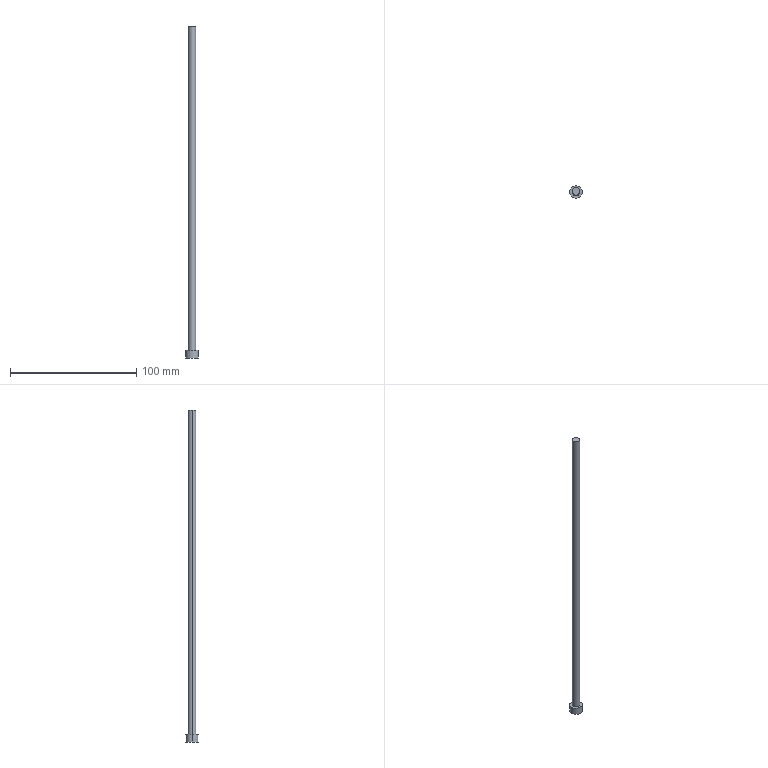Part | Creo | 1 solid | 7 faces | box 10 x 10 x 263.337 mm | volume 7747 mm3 | cylinder 4 | plane 3 | commonest cylinder face diameters 6 x2 10 x2
STEP:
#1=CARTESIAN_POINT('',(5.,161.,-32.663));
#2=VERTEX_POINT('',#1);
#3=CARTESIAN_POINT('',(11.,161.,-32.663));
#4=VERTEX_POINT('',#3);
#5=CARTESIAN_POINT('',(8.,161.,-32.663));
#6=DIRECTION('',(0.,0.,1.));
#7=DIRECTION('',(-1.,0.,0.));
#8=AXIS2_PLACEMENT_3D('',#5,#6,#7);
#9=CIRCLE('',#8,3.);
#10=EDGE_CURVE('',#2,#4,#9,.T.);
#11=ORIENTED_EDGE('',*,*,#10,.F.);
#12=CARTESIAN_POINT('',(8.,161.,-32.663));
#13=DIRECTION('',(0.,0.,1.));
#14=DIRECTION('',(1.,0.,0.));
#15=AXIS2_PLACEMENT_3D('',#12,#13,#14);
#16=CIRCLE('',#15,3.);
#17=EDGE_CURVE('',#4,#2,#16,.T.);
#18=ORIENTED_EDGE('',*,*,#17,.F.);
#19=EDGE_LOOP('',(#11,#18));
#20=FACE_OUTER_BOUND('',#19,.F.);
#21=CARTESIAN_POINT('',(-0.00000969,166.325,-32.663));
#22=DIRECTION('',(0.,0.,-1.));
#23=DIRECTION('',(0.,-1.,0.));
#24=AXIS2_PLACEMENT_3D('',#21,#22,#23);
#25=PLANE('',#24);
#26=ADVANCED_FACE('',(#20),#25,.F.);
#27=CARTESIAN_POINT('',(11.,161.,-290.));
#28=VERTEX_POINT('',#27);
#29=CARTESIAN_POINT('',(5.,161.,-290.));
#30=VERTEX_POINT('',#29);
#31=CARTESIAN_POINT('',(8.,161.,-290.));
#32=DIRECTION('',(0.,0.,-1.));
#33=DIRECTION('',(1.,0.,0.));
#34=AXIS2_PLACEMENT_3D('',#31,#32,#33);
#35=CIRCLE('',#34,3.);
#36=EDGE_CURVE('',#28,#30,#35,.T.);
#37=ORIENTED_EDGE('',*,*,#36,.T.);
#38=CARTESIAN_POINT('',(5.,161.,-290.));
#39=DIRECTION('',(0.,0.,1.));
#40=VECTOR('',#39,257.337);
#41=LINE('',#38,#40);
#42=EDGE_CURVE('',#30,#2,#41,.T.);
#43=ORIENTED_EDGE('',*,*,#42,.T.);
#44=ORIENTED_EDGE('',*,*,#10,.T.);
#45=CARTESIAN_POINT('',(11.,161.,-290.));
#46=DIRECTION('',(0.,0.,1.));
#47=VECTOR('',#46,257.337);
#48=LINE('',#45,#47);
#49=EDGE_CURVE('',#28,#4,#48,.T.);
#50=ORIENTED_EDGE('',*,*,#49,.F.);
#51=EDGE_LOOP('',(#37,#43,#44,#50));
#52=FACE_OUTER_BOUND('',#51,.F.);
#53=CARTESIAN_POINT('',(8.,161.,-351.071));
#54=DIRECTION('',(0.,0.,1.));
#55=DIRECTION('',(-1.,0.,0.));
#56=AXIS2_PLACEMENT_3D('',#53,#54,#55);
#57=CYLINDRICAL_SURFACE('',#56,3.);
#58=ADVANCED_FACE('',(#52),#57,.T.);
#59=CARTESIAN_POINT('',(13.,161.,-290.));
#60=VERTEX_POINT('',#59);
#61=CARTESIAN_POINT('',(3.,161.,-290.));
#62=VERTEX_POINT('',#61);
#63=CARTESIAN_POINT('',(8.,161.,-290.));
#64=DIRECTION('',(0.,0.,1.));
#65=DIRECTION('',(1.,0.,0.));
#66=AXIS2_PLACEMENT_3D('',#63,#64,#65);
#67=CIRCLE('',#66,5.);
#68=EDGE_CURVE('',#60,#62,#67,.T.);
#69=ORIENTED_EDGE('',*,*,#68,.F.);
#70=CARTESIAN_POINT('',(8.,161.,-290.));
#71=DIRECTION('',(0.,0.,1.));
#72=DIRECTION('',(-1.,0.,0.));
#73=AXIS2_PLACEMENT_3D('',#70,#71,#72);
#74=CIRCLE('',#73,5.);
#75=EDGE_CURVE('',#62,#60,#74,.T.);
#76=ORIENTED_EDGE('',*,*,#75,.F.);
#77=EDGE_LOOP('',(#69,#76));
#78=FACE_OUTER_BOUND('',#77,.F.);
#79=ORIENTED_EDGE('',*,*,#36,.F.);
#80=CARTESIAN_POINT('',(8.,161.,-290.));
#81=DIRECTION('',(0.,0.,-1.));
#82=DIRECTION('',(-1.,0.,0.));
#83=AXIS2_PLACEMENT_3D('',#80,#81,#82);
#84=CIRCLE('',#83,3.);
#85=EDGE_CURVE('',#30,#28,#84,.T.);
#86=ORIENTED_EDGE('',*,*,#85,.F.);
#87=EDGE_LOOP('',(#79,#86));
#88=FACE_BOUND('',#87,.F.);
#89=CARTESIAN_POINT('',(8.,161.,-290.));
#90=DIRECTION('',(0.,0.,1.));
#91=DIRECTION('',(-1.,0.,0.));
#92=AXIS2_PLACEMENT_3D('',#89,#90,#91);
#93=PLANE('',#92);
#94=ADVANCED_FACE('',(#78,#88),#93,.T.);
#95=ORIENTED_EDGE('',*,*,#85,.T.);
#96=ORIENTED_EDGE('',*,*,#49,.T.);
#97=ORIENTED_EDGE('',*,*,#17,.T.);
#98=ORIENTED_EDGE('',*,*,#42,.F.);
#99=EDGE_LOOP('',(#95,#96,#97,#98));
#100=FACE_OUTER_BOUND('',#99,.F.);
#101=CARTESIAN_POINT('',(8.,161.,-351.071));
#102=DIRECTION('',(0.,0.,1.));
#103=DIRECTION('',(-1.,0.,0.));
#104=AXIS2_PLACEMENT_3D('',#101,#102,#103);
#105=CYLINDRICAL_SURFACE('',#104,3.);
#106=ADVANCED_FACE('',(#100),#105,.T.);
#107=ORIENTED_EDGE('',*,*,#68,.T.);
#108=CARTESIAN_POINT('',(3.,161.,-296.));
#109=VERTEX_POINT('',#108);
#110=CARTESIAN_POINT('',(3.,161.,-296.));
#111=DIRECTION('',(0.,0.,1.));
#112=VECTOR('',#111,6.);
#113=LINE('',#110,#112);
#114=EDGE_CURVE('',#109,#62,#113,.T.);
#115=ORIENTED_EDGE('',*,*,#114,.F.);
#116=CARTESIAN_POINT('',(13.,161.,-296.));
#117=VERTEX_POINT('',#116);
#118=CARTESIAN_POINT('',(8.,161.,-296.));
#119=DIRECTION('',(0.,0.,-1.));
#120=DIRECTION('',(-1.,0.,0.));
#121=AXIS2_PLACEMENT_3D('',#118,#119,#120);
#122=CIRCLE('',#121,5.);
#123=EDGE_CURVE('',#109,#117,#122,.T.);
#124=ORIENTED_EDGE('',*,*,#123,.T.);
#125=CARTESIAN_POINT('',(13.,161.,-296.));
#126=DIRECTION('',(0.,0.,1.));
#127=VECTOR('',#126,6.);
#128=LINE('',#125,#127);
#129=EDGE_CURVE('',#117,#60,#128,.T.);
#130=ORIENTED_EDGE('',*,*,#129,.T.);
#131=EDGE_LOOP('',(#107,#115,#124,#130));
#132=FACE_OUTER_BOUND('',#131,.F.);
#133=CARTESIAN_POINT('',(8.,161.,-296.));
#134=DIRECTION('',(0.,0.,1.));
#135=DIRECTION('',(-1.,0.,0.));
#136=AXIS2_PLACEMENT_3D('',#133,#134,#135);
#137=CYLINDRICAL_SURFACE('',#136,5.);
#138=ADVANCED_FACE('',(#132),#137,.T.);
#139=ORIENTED_EDGE('',*,*,#75,.T.);
#140=ORIENTED_EDGE('',*,*,#129,.F.);
#141=CARTESIAN_POINT('',(8.,161.,-296.));
#142=DIRECTION('',(0.,0.,-1.));
#143=DIRECTION('',(1.,0.,0.));
#144=AXIS2_PLACEMENT_3D('',#141,#142,#143);
#145=CIRCLE('',#144,5.);
#146=EDGE_CURVE('',#117,#109,#145,.T.);
#147=ORIENTED_EDGE('',*,*,#146,.T.);
#148=ORIENTED_EDGE('',*,*,#114,.T.);
#149=EDGE_LOOP('',(#139,#140,#147,#148));
#150=FACE_OUTER_BOUND('',#149,.F.);
#151=CARTESIAN_POINT('',(8.,161.,-296.));
#152=DIRECTION('',(0.,0.,1.));
#153=DIRECTION('',(-1.,0.,0.));
#154=AXIS2_PLACEMENT_3D('',#151,#152,#153);
#155=CYLINDRICAL_SURFACE('',#154,5.);
#156=ADVANCED_FACE('',(#150),#155,.T.);
#157=ORIENTED_EDGE('',*,*,#146,.F.);
#158=ORIENTED_EDGE('',*,*,#123,.F.);
#159=EDGE_LOOP('',(#157,#158));
#160=FACE_OUTER_BOUND('',#159,.F.);
#161=CARTESIAN_POINT('',(10.,0.4953,-296.));
#162=DIRECTION('',(0.,0.,1.));
#163=DIRECTION('',(0.,1.,0.));
#164=AXIS2_PLACEMENT_3D('',#161,#162,#163);
#165=PLANE('',#164);
#166=ADVANCED_FACE('',(#160),#165,.F.);
#167=CLOSED_SHELL('',(#26,#58,#94,#106,#138,#156,#166));
#168=MANIFOLD_SOLID_BREP('',#167);
#169=(LENGTH_UNIT()NAMED_UNIT(*)SI_UNIT(.MILLI.,.METRE.));
#170=UNCERTAINTY_MEASURE_WITH_UNIT(LENGTH_MEASURE(0.02637),#169,'','');
#171=(NAMED_UNIT(*)PLANE_ANGLE_UNIT()SI_UNIT($,.RADIAN.));
#172=PLANE_ANGLE_MEASURE_WITH_UNIT(PLANE_ANGLE_MEASURE(0.01745),#171);
#173=(CONVERSION_BASED_UNIT('DEGREE',#172)NAMED_UNIT(*)PLANE_ANGLE_UNIT());
#174=(NAMED_UNIT(*)SI_UNIT($,.STERADIAN.)SOLID_ANGLE_UNIT());
#175=(GEOMETRIC_REPRESENTATION_CONTEXT(3)GLOBAL_UNCERTAINTY_ASSIGNED_CONTEXT((#170))GLOBAL_UNIT_ASSIGNED_CONTEXT((#169,#173,#174))REPRESENTATION_CONTEXT('',''));
#176=ADVANCED_BREP_SHAPE_REPRESENTATION('',(#168),#175);